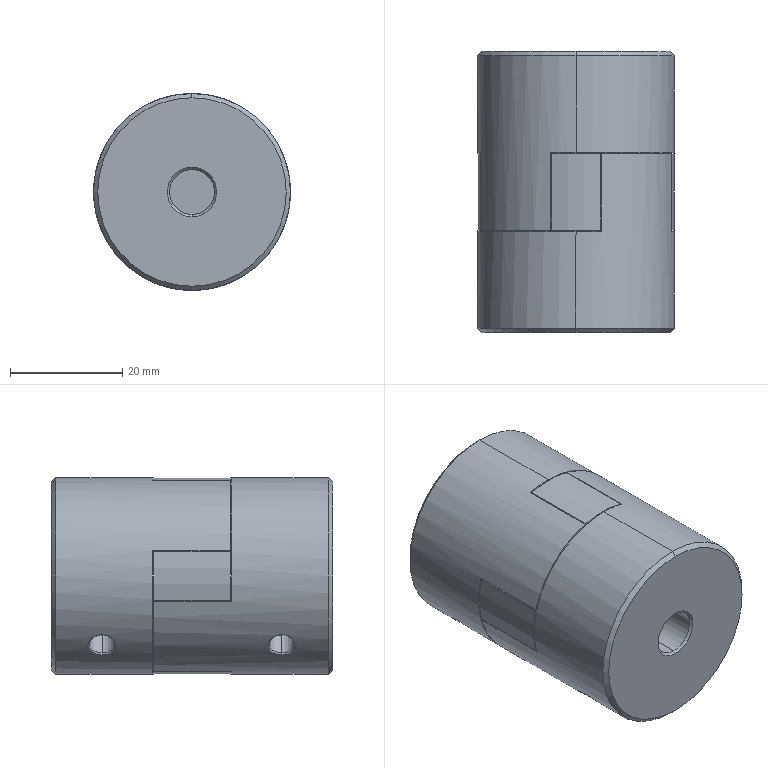Part | STEP file | MJ45 coupling | 3 solids | 85 faces | box 35 x 50 x 35 mm | volume 41891 mm3 | cylinder 41 | plane 28 | cone 8 | spline 8 | commonest cylinder face diameters 35 x9 0.5 x8 4.5 x8 26 x8 8 x4 21 x4